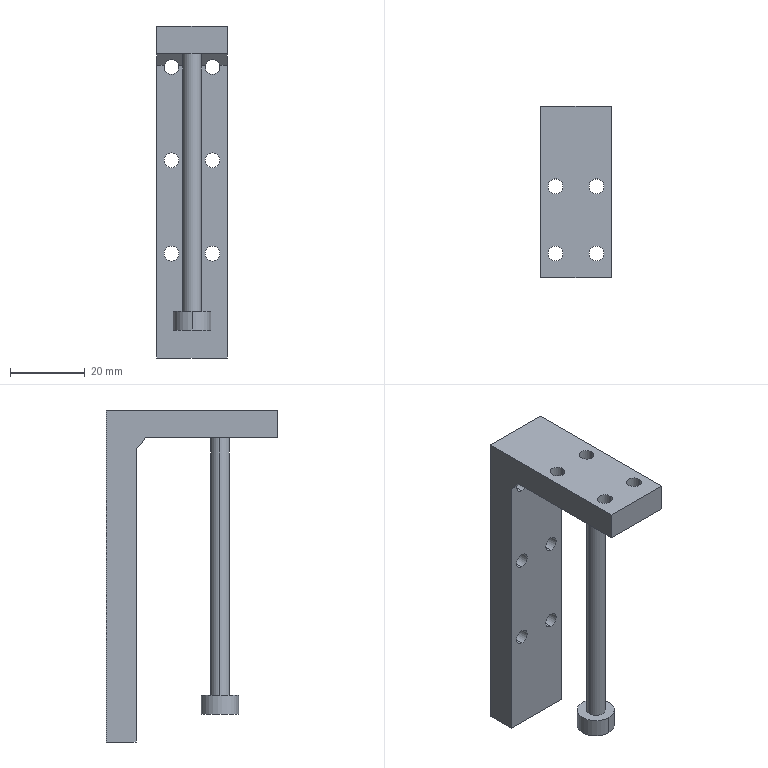Part | NX | 1 solid | 35 faces | box 19 x 46 x 89 mm | volume 19778 mm3 | cylinder 24 | plane 11 | commonest cylinder face diameters 4 x20 5 x2 10 x2
STEP:
#1=CARTESIAN_POINT('',(0.,-5.,-81.5));
#2=VERTEX_POINT('',#1);
#3=CARTESIAN_POINT('',(0.,5.,-81.5));
#4=VERTEX_POINT('',#3);
#5=CARTESIAN_POINT('',(0.,0.,-81.5));
#6=DIRECTION('',(0.,0.,-1.));
#7=DIRECTION('',(0.,1.,0.));
#8=AXIS2_PLACEMENT_3D('',#5,#6,#7);
#9=CIRCLE('',#8,5.);
#10=EDGE_CURVE('',#2,#4,#9,.T.);
#11=ORIENTED_EDGE('',*,*,#10,.F.);
#12=CARTESIAN_POINT('',(0.,-5.,-76.5));
#13=VERTEX_POINT('',#12);
#14=CARTESIAN_POINT('',(0.,-5.,-81.5));
#15=DIRECTION('',(0.,0.,1.));
#16=VECTOR('',#15,1000.);
#17=LINE('',#14,#16);
#18=EDGE_CURVE('',#13,#2,#17,.F.);
#19=ORIENTED_EDGE('',*,*,#18,.F.);
#20=CARTESIAN_POINT('',(0.,5.,-76.5));
#21=VERTEX_POINT('',#20);
#22=CARTESIAN_POINT('',(0.,0.,-76.5));
#23=DIRECTION('',(0.,0.,-1.));
#24=DIRECTION('',(0.,1.,0.));
#25=AXIS2_PLACEMENT_3D('',#22,#23,#24);
#26=CIRCLE('',#25,5.);
#27=EDGE_CURVE('',#13,#21,#26,.T.);
#28=ORIENTED_EDGE('',*,*,#27,.T.);
#29=CARTESIAN_POINT('',(0.,5.,-81.5));
#30=DIRECTION('',(0.,0.,1.));
#31=VECTOR('',#30,1000.);
#32=LINE('',#29,#31);
#33=EDGE_CURVE('',#21,#4,#32,.F.);
#34=ORIENTED_EDGE('',*,*,#33,.T.);
#35=EDGE_LOOP('',(#11,#19,#28,#34));
#36=FACE_BOUND('',#35,.T.);
#37=CARTESIAN_POINT('',(0.,0.,-81.5));
#38=DIRECTION('',(0.,0.,1.));
#39=DIRECTION('',(0.,-1.,0.));
#40=AXIS2_PLACEMENT_3D('',#37,#38,#39);
#41=CYLINDRICAL_SURFACE('',#40,5.);
#42=ADVANCED_FACE('',(#36),#41,.T.);
#43=CARTESIAN_POINT('',(-5.5,30.5,-59.));
#44=VERTEX_POINT('',#43);
#45=CARTESIAN_POINT('',(-5.5,30.5,-63.));
#46=VERTEX_POINT('',#45);
#47=CARTESIAN_POINT('',(-5.5,30.5,-61.));
#48=DIRECTION('',(0.,1.,0.));
#49=DIRECTION('',(0.,0.,1.));
#50=AXIS2_PLACEMENT_3D('',#47,#48,#49);
#51=CIRCLE('',#50,2.);
#52=EDGE_CURVE('',#44,#46,#51,.T.);
#53=ORIENTED_EDGE('',*,*,#52,.T.);
#54=CARTESIAN_POINT('',(-5.5,22.5,-63.));
#55=VERTEX_POINT('',#54);
#56=CARTESIAN_POINT('',(-5.5,-15.5,-63.));
#57=DIRECTION('',(0.,1.,0.));
#58=VECTOR('',#57,1000.);
#59=LINE('',#56,#58);
#60=EDGE_CURVE('',#46,#55,#59,.F.);
#61=ORIENTED_EDGE('',*,*,#60,.T.);
#62=CARTESIAN_POINT('',(-5.5,22.5,-59.));
#63=VERTEX_POINT('',#62);
#64=CARTESIAN_POINT('',(-5.5,22.5,-61.));
#65=DIRECTION('',(0.,1.,0.));
#66=DIRECTION('',(0.,0.,1.));
#67=AXIS2_PLACEMENT_3D('',#64,#65,#66);
#68=CIRCLE('',#67,2.);
#69=EDGE_CURVE('',#63,#55,#68,.T.);
#70=ORIENTED_EDGE('',*,*,#69,.F.);
#71=CARTESIAN_POINT('',(-5.5,-15.5,-59.));
#72=DIRECTION('',(0.,1.,0.));
#73=VECTOR('',#72,1000.);
#74=LINE('',#71,#73);
#75=EDGE_CURVE('',#44,#63,#74,.F.);
#76=ORIENTED_EDGE('',*,*,#75,.F.);
#77=EDGE_LOOP('',(#53,#61,#70,#76));
#78=FACE_BOUND('',#77,.T.);
#79=CARTESIAN_POINT('',(-5.5,-15.5,-61.));
#80=DIRECTION('',(0.,1.,0.));
#81=DIRECTION('',(0.,0.,1.));
#82=AXIS2_PLACEMENT_3D('',#79,#80,#81);
#83=CYLINDRICAL_SURFACE('',#82,2.);
#84=ADVANCED_FACE('',(#78),#83,.F.);
#85=CARTESIAN_POINT('',(5.5,30.5,-63.));
#86=VERTEX_POINT('',#85);
#87=CARTESIAN_POINT('',(5.5,30.5,-59.));
#88=VERTEX_POINT('',#87);
#89=CARTESIAN_POINT('',(5.5,30.5,-61.));
#90=DIRECTION('',(0.,1.,0.));
#91=DIRECTION('',(0.,0.,1.));
#92=AXIS2_PLACEMENT_3D('',#89,#90,#91);
#93=CIRCLE('',#92,2.);
#94=EDGE_CURVE('',#86,#88,#93,.T.);
#95=ORIENTED_EDGE('',*,*,#94,.T.);
#96=CARTESIAN_POINT('',(5.5,22.5,-59.));
#97=VERTEX_POINT('',#96);
#98=CARTESIAN_POINT('',(5.5,-15.5,-59.));
#99=DIRECTION('',(0.,1.,0.));
#100=VECTOR('',#99,1000.);
#101=LINE('',#98,#100);
#102=EDGE_CURVE('',#97,#88,#101,.T.);
#103=ORIENTED_EDGE('',*,*,#102,.F.);
#104=CARTESIAN_POINT('',(5.5,22.5,-63.));
#105=VERTEX_POINT('',#104);
#106=CARTESIAN_POINT('',(5.5,22.5,-61.));
#107=DIRECTION('',(0.,1.,0.));
#108=DIRECTION('',(0.,0.,1.));
#109=AXIS2_PLACEMENT_3D('',#106,#107,#108);
#110=CIRCLE('',#109,2.);
#111=EDGE_CURVE('',#105,#97,#110,.T.);
#112=ORIENTED_EDGE('',*,*,#111,.F.);
#113=CARTESIAN_POINT('',(5.5,-15.5,-63.));
#114=DIRECTION('',(0.,1.,0.));
#115=VECTOR('',#114,1000.);
#116=LINE('',#113,#115);
#117=EDGE_CURVE('',#105,#86,#116,.T.);
#118=ORIENTED_EDGE('',*,*,#117,.T.);
#119=EDGE_LOOP('',(#95,#103,#112,#118));
#120=FACE_BOUND('',#119,.T.);
#121=CARTESIAN_POINT('',(5.5,-15.5,-61.));
#122=DIRECTION('',(0.,1.,0.));
#123=DIRECTION('',(0.,0.,1.));
#124=AXIS2_PLACEMENT_3D('',#121,#122,#123);
#125=CYLINDRICAL_SURFACE('',#124,2.);
#126=ADVANCED_FACE('',(#120),#125,.F.);
#127=CARTESIAN_POINT('',(5.5,22.5,-13.));
#128=VERTEX_POINT('',#127);
#129=CARTESIAN_POINT('',(3.564,22.5,-10.5));
#130=VERTEX_POINT('',#129);
#131=CARTESIAN_POINT('',(5.5,22.5,-11.));
#132=DIRECTION('',(0.,1.,0.));
#133=DIRECTION('',(0.,0.,1.));
#134=AXIS2_PLACEMENT_3D('',#131,#132,#133);
#135=CIRCLE('',#134,2.);
#136=EDGE_CURVE('',#128,#130,#135,.T.);
#137=ORIENTED_EDGE('',*,*,#136,.F.);
#138=CARTESIAN_POINT('',(5.5,30.5,-13.));
#139=VERTEX_POINT('',#138);
#140=CARTESIAN_POINT('',(5.5,-15.5,-13.));
#141=DIRECTION('',(0.,1.,0.));
#142=VECTOR('',#141,1000.);
#143=LINE('',#140,#142);
#144=EDGE_CURVE('',#139,#128,#143,.F.);
#145=ORIENTED_EDGE('',*,*,#144,.F.);
#146=CARTESIAN_POINT('',(5.5,30.5,-9.));
#147=VERTEX_POINT('',#146);
#148=CARTESIAN_POINT('',(5.5,30.5,-11.));
#149=DIRECTION('',(0.,1.,0.));
#150=DIRECTION('',(0.,0.,-1.));
#151=AXIS2_PLACEMENT_3D('',#148,#149,#150);
#152=CIRCLE('',#151,2.);
#153=EDGE_CURVE('',#139,#147,#152,.T.);
#154=ORIENTED_EDGE('',*,*,#153,.T.);
#155=CARTESIAN_POINT('',(5.5,21.241,-9.));
#156=VERTEX_POINT('',#155);
#157=CARTESIAN_POINT('',(5.5,-15.5,-9.));
#158=DIRECTION('',(0.,1.,0.));
#159=VECTOR('',#158,1000.);
#160=LINE('',#157,#159);
#161=EDGE_CURVE('',#147,#156,#160,.F.);
#162=ORIENTED_EDGE('',*,*,#161,.T.);
#163=CARTESIAN_POINT('',(3.564,22.5,-10.5));
#164=CARTESIAN_POINT('',(3.801,21.729,-9.581));
#165=CARTESIAN_POINT('',(4.551,21.241,-9.));
#166=CARTESIAN_POINT('',(5.5,21.241,-9.));
#167=(BOUNDED_CURVE()B_SPLINE_CURVE(3,(#163,#164,#165,#166),.UNSPECIFIED.,.F.,.F.)B_SPLINE_CURVE_WITH_KNOTS((4,4),(1.823,3.142),.UNSPECIFIED.)CURVE()GEOMETRIC_REPRESENTATION_ITEM()RATIONAL_B_SPLINE_CURVE((1.,0.8604,0.8604,1.))REPRESENTATION_ITEM(''));
#168=EDGE_CURVE('',#130,#156,#167,.T.);
#169=ORIENTED_EDGE('',*,*,#168,.F.);
#170=EDGE_LOOP('',(#137,#145,#154,#162,#169));
#171=FACE_BOUND('',#170,.T.);
#172=CARTESIAN_POINT('',(5.5,-15.5,-11.));
#173=DIRECTION('',(0.,1.,0.));
#174=DIRECTION('',(0.,0.,1.));
#175=AXIS2_PLACEMENT_3D('',#172,#173,#174);
#176=CYLINDRICAL_SURFACE('',#175,2.);
#177=ADVANCED_FACE('',(#171),#176,.F.);
#178=CARTESIAN_POINT('',(-5.5,22.5,-38.));
#179=VERTEX_POINT('',#178);
#180=CARTESIAN_POINT('',(-5.5,22.5,-34.));
#181=VERTEX_POINT('',#180);
#182=CARTESIAN_POINT('',(-5.5,22.5,-36.));
#183=DIRECTION('',(0.,1.,0.));
#184=DIRECTION('',(0.,0.,1.));
#185=AXIS2_PLACEMENT_3D('',#182,#183,#184);
#186=CIRCLE('',#185,2.);
#187=EDGE_CURVE('',#179,#181,#186,.T.);
#188=ORIENTED_EDGE('',*,*,#187,.F.);
#189=CARTESIAN_POINT('',(-5.5,30.5,-38.));
#190=VERTEX_POINT('',#189);
#191=CARTESIAN_POINT('',(-5.5,-15.5,-38.));
#192=DIRECTION('',(0.,1.,0.));
#193=VECTOR('',#192,1000.);
#194=LINE('',#191,#193);
#195=EDGE_CURVE('',#190,#179,#194,.F.);
#196=ORIENTED_EDGE('',*,*,#195,.F.);
#197=CARTESIAN_POINT('',(-5.5,30.5,-34.));
#198=VERTEX_POINT('',#197);
#199=CARTESIAN_POINT('',(-5.5,30.5,-36.));
#200=DIRECTION('',(0.,1.,0.));
#201=DIRECTION('',(0.,0.,1.));
#202=AXIS2_PLACEMENT_3D('',#199,#200,#201);
#203=CIRCLE('',#202,2.);
#204=EDGE_CURVE('',#190,#198,#203,.T.);
#205=ORIENTED_EDGE('',*,*,#204,.T.);
#206=CARTESIAN_POINT('',(-5.5,-15.5,-34.));
#207=DIRECTION('',(0.,1.,0.));
#208=VECTOR('',#207,1000.);
#209=LINE('',#206,#208);
#210=EDGE_CURVE('',#198,#181,#209,.F.);
#211=ORIENTED_EDGE('',*,*,#210,.T.);
#212=EDGE_LOOP('',(#188,#196,#205,#211));
#213=FACE_BOUND('',#212,.T.);
#214=CARTESIAN_POINT('',(-5.5,-15.5,-36.));
#215=DIRECTION('',(0.,1.,0.));
#216=DIRECTION('',(0.,0.,1.));
#217=AXIS2_PLACEMENT_3D('',#214,#215,#216);
#218=CYLINDRICAL_SURFACE('',#217,2.);
#219=ADVANCED_FACE('',(#213),#218,.F.);
#220=CARTESIAN_POINT('',(-5.5,22.5,-13.));
#221=VERTEX_POINT('',#220);
#222=CARTESIAN_POINT('',(-7.436,22.5,-10.5));
#223=VERTEX_POINT('',#222);
#224=CARTESIAN_POINT('',(-5.5,22.5,-11.));
#225=DIRECTION('',(0.,1.,0.));
#226=DIRECTION('',(0.,0.,1.));
#227=AXIS2_PLACEMENT_3D('',#224,#225,#226);
#228=CIRCLE('',#227,2.);
#229=EDGE_CURVE('',#221,#223,#228,.T.);
#230=ORIENTED_EDGE('',*,*,#229,.F.);
#231=CARTESIAN_POINT('',(-5.5,30.5,-13.));
#232=VERTEX_POINT('',#231);
#233=CARTESIAN_POINT('',(-5.5,-15.5,-13.));
#234=DIRECTION('',(0.,1.,0.));
#235=VECTOR('',#234,1000.);
#236=LINE('',#233,#235);
#237=EDGE_CURVE('',#232,#221,#236,.F.);
#238=ORIENTED_EDGE('',*,*,#237,.F.);
#239=CARTESIAN_POINT('',(-5.5,30.5,-9.));
#240=VERTEX_POINT('',#239);
#241=CARTESIAN_POINT('',(-5.5,30.5,-11.));
#242=DIRECTION('',(0.,1.,0.));
#243=DIRECTION('',(0.,0.,1.));
#244=AXIS2_PLACEMENT_3D('',#241,#242,#243);
#245=CIRCLE('',#244,2.);
#246=EDGE_CURVE('',#232,#240,#245,.T.);
#247=ORIENTED_EDGE('',*,*,#246,.T.);
#248=CARTESIAN_POINT('',(-5.5,21.241,-9.));
#249=VERTEX_POINT('',#248);
#250=CARTESIAN_POINT('',(-5.5,-15.5,-9.));
#251=DIRECTION('',(0.,1.,0.));
#252=VECTOR('',#251,1000.);
#253=LINE('',#250,#252);
#254=EDGE_CURVE('',#240,#249,#253,.F.);
#255=ORIENTED_EDGE('',*,*,#254,.T.);
#256=CARTESIAN_POINT('',(-7.436,22.5,-10.5));
#257=CARTESIAN_POINT('',(-7.199,21.729,-9.581));
#258=CARTESIAN_POINT('',(-6.449,21.241,-9.));
#259=CARTESIAN_POINT('',(-5.5,21.241,-9.));
#260=(BOUNDED_CURVE()B_SPLINE_CURVE(3,(#256,#257,#258,#259),.UNSPECIFIED.,.F.,.F.)B_SPLINE_CURVE_WITH_KNOTS((4,4),(1.823,3.142),.UNSPECIFIED.)CURVE()GEOMETRIC_REPRESENTATION_ITEM()RATIONAL_B_SPLINE_CURVE((1.,0.8604,0.8604,1.))REPRESENTATION_ITEM(''));
#261=EDGE_CURVE('',#223,#249,#260,.T.);
#262=ORIENTED_EDGE('',*,*,#261,.F.);
#263=EDGE_LOOP('',(#230,#238,#247,#255,#262));
#264=FACE_BOUND('',#263,.T.);
#265=CARTESIAN_POINT('',(-5.5,-15.5,-11.));
#266=DIRECTION('',(0.,1.,0.));
#267=DIRECTION('',(0.,0.,1.));
#268=AXIS2_PLACEMENT_3D('',#265,#266,#267);
#269=CYLINDRICAL_SURFACE('',#268,2.);
#270=ADVANCED_FACE('',(#264),#269,.F.);
#271=CARTESIAN_POINT('',(5.5,30.5,-38.));
#272=VERTEX_POINT('',#271);
#273=CARTESIAN_POINT('',(5.5,30.5,-34.));
#274=VERTEX_POINT('',#273);
#275=CARTESIAN_POINT('',(5.5,30.5,-36.));
#276=DIRECTION('',(0.,1.,0.));
#277=DIRECTION('',(0.,0.,-1.));
#278=AXIS2_PLACEMENT_3D('',#275,#276,#277);
#279=CIRCLE('',#278,2.);
#280=EDGE_CURVE('',#272,#274,#279,.T.);
#281=ORIENTED_EDGE('',*,*,#280,.T.);
#282=CARTESIAN_POINT('',(5.5,22.5,-34.));
#283=VERTEX_POINT('',#282);
#284=CARTESIAN_POINT('',(5.5,-15.5,-34.));
#285=DIRECTION('',(0.,1.,0.));
#286=VECTOR('',#285,1000.);
#287=LINE('',#284,#286);
#288=EDGE_CURVE('',#283,#274,#287,.T.);
#289=ORIENTED_EDGE('',*,*,#288,.F.);
#290=CARTESIAN_POINT('',(5.5,22.5,-38.));
#291=VERTEX_POINT('',#290);
#292=CARTESIAN_POINT('',(5.5,22.5,-36.));
#293=DIRECTION('',(0.,1.,0.));
#294=DIRECTION('',(0.,0.,1.));
#295=AXIS2_PLACEMENT_3D('',#292,#293,#294);
#296=CIRCLE('',#295,2.);
#297=EDGE_CURVE('',#291,#283,#296,.T.);
#298=ORIENTED_EDGE('',*,*,#297,.F.);
#299=CARTESIAN_POINT('',(5.5,-15.5,-38.));
#300=DIRECTION('',(0.,1.,0.));
#301=VECTOR('',#300,1000.);
#302=LINE('',#299,#301);
#303=EDGE_CURVE('',#291,#272,#302,.T.);
#304=ORIENTED_EDGE('',*,*,#303,.T.);
#305=EDGE_LOOP('',(#281,#289,#298,#304));
#306=FACE_BOUND('',#305,.T.);
#307=CARTESIAN_POINT('',(5.5,-15.5,-36.));
#308=DIRECTION('',(0.,1.,0.));
#309=DIRECTION('',(0.,0.,1.));
#310=AXIS2_PLACEMENT_3D('',#307,#308,#309);
#311=CYLINDRICAL_SURFACE('',#310,2.);
#312=ADVANCED_FACE('',(#306),#311,.F.);
#313=CARTESIAN_POINT('',(3.5,-9.,-7.5));
#314=VERTEX_POINT('',#313);
#315=CARTESIAN_POINT('',(7.5,-9.,-7.5));
#316=VERTEX_POINT('',#315);
#317=CARTESIAN_POINT('',(5.5,-9.,-7.5));
#318=DIRECTION('',(0.,0.,1.));
#319=DIRECTION('',(0.,-1.,0.));
#320=AXIS2_PLACEMENT_3D('',#317,#318,#319);
#321=CIRCLE('',#320,2.);
#322=EDGE_CURVE('',#314,#316,#321,.T.);
#323=ORIENTED_EDGE('',*,*,#322,.F.);
#324=CARTESIAN_POINT('',(3.5,-9.,0.));
#325=VERTEX_POINT('',#324);
#326=CARTESIAN_POINT('',(3.5,-9.,-89.));
#327=DIRECTION('',(0.,0.,1.));
#328=VECTOR('',#327,1000.);
#329=LINE('',#326,#328);
#330=EDGE_CURVE('',#314,#325,#329,.T.);
#331=ORIENTED_EDGE('',*,*,#330,.T.);
#332=CARTESIAN_POINT('',(7.5,-9.,0.));
#333=VERTEX_POINT('',#332);
#334=CARTESIAN_POINT('',(5.5,-9.,0.));
#335=DIRECTION('',(0.,0.,1.));
#336=DIRECTION('',(-1.,0.,0.));
#337=AXIS2_PLACEMENT_3D('',#334,#335,#336);
#338=CIRCLE('',#337,2.);
#339=EDGE_CURVE('',#325,#333,#338,.T.);
#340=ORIENTED_EDGE('',*,*,#339,.T.);
#341=CARTESIAN_POINT('',(7.5,-9.,-89.));
#342=DIRECTION('',(0.,0.,1.));
#343=VECTOR('',#342,1000.);
#344=LINE('',#341,#343);
#345=EDGE_CURVE('',#316,#333,#344,.T.);
#346=ORIENTED_EDGE('',*,*,#345,.F.);
#347=EDGE_LOOP('',(#323,#331,#340,#346));
#348=FACE_BOUND('',#347,.T.);
#349=CARTESIAN_POINT('',(5.5,-9.,-89.));
#350=DIRECTION('',(0.,0.,1.));
#351=DIRECTION('',(1.,0.,0.));
#352=AXIS2_PLACEMENT_3D('',#349,#350,#351);
#353=CYLINDRICAL_SURFACE('',#352,2.);
#354=ADVANCED_FACE('',(#348),#353,.F.);
#355=CARTESIAN_POINT('',(-7.5,-9.,-7.5));
#356=VERTEX_POINT('',#355);
#357=CARTESIAN_POINT('',(-3.5,-9.,-7.5));
#358=VERTEX_POINT('',#357);
#359=CARTESIAN_POINT('',(-5.5,-9.,-7.5));
#360=DIRECTION('',(0.,0.,1.));
#361=DIRECTION('',(0.,-1.,0.));
#362=AXIS2_PLACEMENT_3D('',#359,#360,#361);
#363=CIRCLE('',#362,2.);
#364=EDGE_CURVE('',#356,#358,#363,.T.);
#365=ORIENTED_EDGE('',*,*,#364,.F.);
#366=CARTESIAN_POINT('',(-7.5,-9.,0.));
#367=VERTEX_POINT('',#366);
#368=CARTESIAN_POINT('',(-7.5,-9.,-89.));
#369=DIRECTION('',(0.,0.,1.));
#370=VECTOR('',#369,1000.);
#371=LINE('',#368,#370);
#372=EDGE_CURVE('',#367,#356,#371,.F.);
#373=ORIENTED_EDGE('',*,*,#372,.F.);
#374=CARTESIAN_POINT('',(-3.5,-9.,0.));
#375=VERTEX_POINT('',#374);
#376=CARTESIAN_POINT('',(-5.5,-9.,0.));
#377=DIRECTION('',(0.,0.,1.));
#378=DIRECTION('',(1.,0.,0.));
#379=AXIS2_PLACEMENT_3D('',#376,#377,#378);
#380=CIRCLE('',#379,2.);
#381=EDGE_CURVE('',#367,#375,#380,.T.);
#382=ORIENTED_EDGE('',*,*,#381,.T.);
#383=CARTESIAN_POINT('',(-3.5,-9.,-89.));
#384=DIRECTION('',(0.,0.,1.));
#385=VECTOR('',#384,1000.);
#386=LINE('',#383,#385);
#387=EDGE_CURVE('',#375,#358,#386,.F.);
#388=ORIENTED_EDGE('',*,*,#387,.T.);
#389=EDGE_LOOP('',(#365,#373,#382,#388));
#390=FACE_BOUND('',#389,.T.);
#391=CARTESIAN_POINT('',(-5.5,-9.,-89.));
#392=DIRECTION('',(0.,0.,1.));
#393=DIRECTION('',(1.,0.,0.));
#394=AXIS2_PLACEMENT_3D('',#391,#392,#393);
#395=CYLINDRICAL_SURFACE('',#394,2.);
#396=ADVANCED_FACE('',(#390),#395,.F.);
#397=CARTESIAN_POINT('',(-3.5,9.,-7.5));
#398=VERTEX_POINT('',#397);
#399=CARTESIAN_POINT('',(-7.5,9.,-7.5));
#400=VERTEX_POINT('',#399);
#401=CARTESIAN_POINT('',(-5.5,9.,-7.5));
#402=DIRECTION('',(0.,0.,1.));
#403=DIRECTION('',(0.,-1.,0.));
#404=AXIS2_PLACEMENT_3D('',#401,#402,#403);
#405=CIRCLE('',#404,2.);
#406=EDGE_CURVE('',#398,#400,#405,.T.);
#407=ORIENTED_EDGE('',*,*,#406,.F.);
#408=CARTESIAN_POINT('',(-3.5,9.,0.));
#409=VERTEX_POINT('',#408);
#410=CARTESIAN_POINT('',(-3.5,9.,-89.));
#411=DIRECTION('',(0.,0.,1.));
#412=VECTOR('',#411,1000.);
#413=LINE('',#410,#412);
#414=EDGE_CURVE('',#398,#409,#413,.T.);
#415=ORIENTED_EDGE('',*,*,#414,.T.);
#416=CARTESIAN_POINT('',(-7.5,9.,0.));
#417=VERTEX_POINT('',#416);
#418=CARTESIAN_POINT('',(-5.5,9.,0.));
#419=DIRECTION('',(0.,0.,1.));
#420=DIRECTION('',(-1.,0.,0.));
#421=AXIS2_PLACEMENT_3D('',#418,#419,#420);
#422=CIRCLE('',#421,2.);
#423=EDGE_CURVE('',#409,#417,#422,.T.);
#424=ORIENTED_EDGE('',*,*,#423,.T.);
#425=CARTESIAN_POINT('',(-7.5,9.,-89.));
#426=DIRECTION('',(0.,0.,1.));
#427=VECTOR('',#426,1000.);
#428=LINE('',#425,#427);
#429=EDGE_CURVE('',#400,#417,#428,.T.);
#430=ORIENTED_EDGE('',*,*,#429,.F.);
#431=EDGE_LOOP('',(#407,#415,#424,#430));
#432=FACE_BOUND('',#431,.T.);
#433=CARTESIAN_POINT('',(-5.5,9.,-89.));
#434=DIRECTION('',(0.,0.,1.));
#435=DIRECTION('',(1.,0.,0.));
#436=AXIS2_PLACEMENT_3D('',#433,#434,#435);
#437=CYLINDRICAL_SURFACE('',#436,2.);
#438=ADVANCED_FACE('',(#432),#437,.F.);
#439=CARTESIAN_POINT('',(3.5,9.,0.));
#440=VERTEX_POINT('',#439);
#441=CARTESIAN_POINT('',(7.5,9.,0.));
#442=VERTEX_POINT('',#441);
#443=CARTESIAN_POINT('',(5.5,9.,0.));
#444=DIRECTION('',(0.,0.,1.));
#445=DIRECTION('',(1.,0.,0.));
#446=AXIS2_PLACEMENT_3D('',#443,#444,#445);
#447=CIRCLE('',#446,2.);
#448=EDGE_CURVE('',#440,#442,#447,.T.);
#449=ORIENTED_EDGE('',*,*,#448,.T.);
#450=CARTESIAN_POINT('',(7.5,9.,-7.5));
#451=VERTEX_POINT('',#450);
#452=CARTESIAN_POINT('',(7.5,9.,-89.));
#453=DIRECTION('',(0.,0.,1.));
#454=VECTOR('',#453,1000.);
#455=LINE('',#452,#454);
#456=EDGE_CURVE('',#451,#442,#455,.T.);
#457=ORIENTED_EDGE('',*,*,#456,.F.);
#458=CARTESIAN_POINT('',(3.5,9.,-7.5));
#459=VERTEX_POINT('',#458);
#460=CARTESIAN_POINT('',(5.5,9.,-7.5));
#461=DIRECTION('',(0.,0.,1.));
#462=DIRECTION('',(0.,-1.,0.));
#463=AXIS2_PLACEMENT_3D('',#460,#461,#462);
#464=CIRCLE('',#463,2.);
#465=EDGE_CURVE('',#459,#451,#464,.T.);
#466=ORIENTED_EDGE('',*,*,#465,.F.);
#467=CARTESIAN_POINT('',(3.5,9.,-89.));
#468=DIRECTION('',(0.,0.,1.));
#469=VECTOR('',#468,1000.);
#470=LINE('',#467,#469);
#471=EDGE_CURVE('',#459,#440,#470,.T.);
#472=ORIENTED_EDGE('',*,*,#471,.T.);
#473=EDGE_LOOP('',(#449,#457,#466,#472));
#474=FACE_BOUND('',#473,.T.);
#475=CARTESIAN_POINT('',(5.5,9.,-89.));
#476=DIRECTION('',(0.,0.,1.));
#477=DIRECTION('',(1.,0.,0.));
#478=AXIS2_PLACEMENT_3D('',#475,#476,#477);
#479=CYLINDRICAL_SURFACE('',#478,2.);
#480=ADVANCED_FACE('',(#474),#479,.F.);
#481=CARTESIAN_POINT('',(-2.5,0.,-76.5));
#482=VERTEX_POINT('',#481);
#483=CARTESIAN_POINT('',(2.5,0.,-76.5));
#484=VERTEX_POINT('',#483);
#485=CARTESIAN_POINT('',(0.,0.,-76.5));
#486=DIRECTION('',(0.,0.,-1.));
#487=DIRECTION('',(0.,1.,0.));
#488=AXIS2_PLACEMENT_3D('',#485,#486,#487);
#489=CIRCLE('',#488,2.5);
#490=EDGE_CURVE('',#482,#484,#489,.T.);
#491=ORIENTED_EDGE('',*,*,#490,.F.);
#492=CARTESIAN_POINT('',(-2.5,0.,-7.5));
#493=VERTEX_POINT('',#492);
#494=CARTESIAN_POINT('',(-2.5,0.,-79.));
#495=DIRECTION('',(0.,0.,1.));
#496=VECTOR('',#495,1000.);
#497=LINE('',#494,#496);
#498=EDGE_CURVE('',#482,#493,#497,.T.);
#499=ORIENTED_EDGE('',*,*,#498,.T.);
#500=CARTESIAN_POINT('',(2.5,0.,-7.5));
#501=VERTEX_POINT('',#500);
#502=CARTESIAN_POINT('',(0.,0.,-7.5));
#503=DIRECTION('',(0.,0.,-1.));
#504=DIRECTION('',(0.,-1.,0.));
#505=AXIS2_PLACEMENT_3D('',#502,#503,#504);
#506=CIRCLE('',#505,2.5);
#507=EDGE_CURVE('',#493,#501,#506,.T.);
#508=ORIENTED_EDGE('',*,*,#507,.T.);
#509=CARTESIAN_POINT('',(2.5,0.,-79.));
#510=DIRECTION('',(0.,0.,1.));
#511=VECTOR('',#510,1000.);
#512=LINE('',#509,#511);
#513=EDGE_CURVE('',#484,#501,#512,.T.);
#514=ORIENTED_EDGE('',*,*,#513,.F.);
#515=EDGE_LOOP('',(#491,#499,#508,#514));
#516=FACE_BOUND('',#515,.T.);
#517=CARTESIAN_POINT('',(0.,0.,-79.));
#518=DIRECTION('',(0.,0.,1.));
#519=DIRECTION('',(1.,0.,0.));
#520=AXIS2_PLACEMENT_3D('',#517,#518,#519);
#521=CYLINDRICAL_SURFACE('',#520,2.5);
#522=ADVANCED_FACE('',(#516),#521,.T.);
#523=ORIENTED_EDGE('',*,*,#10,.T.);
#524=CARTESIAN_POINT('',(0.,0.,-81.5));
#525=DIRECTION('',(0.,0.,-1.));
#526=DIRECTION('',(0.,1.,0.));
#527=AXIS2_PLACEMENT_3D('',#524,#525,#526);
#528=CIRCLE('',#527,5.);
#529=EDGE_CURVE('',#4,#2,#528,.T.);
#530=ORIENTED_EDGE('',*,*,#529,.T.);
#531=EDGE_LOOP('',(#523,#530));
#532=FACE_BOUND('',#531,.T.);
#533=CARTESIAN_POINT('',(0.,0.,-81.5));
#534=DIRECTION('',(0.,0.,-1.));
#535=DIRECTION('',(-1.,0.,0.));
#536=AXIS2_PLACEMENT_3D('',#533,#534,#535);
#537=PLANE('',#536);
#538=ADVANCED_FACE('',(#532),#537,.T.);
#539=CARTESIAN_POINT('',(-9.5,-15.5,-7.5));
#540=VERTEX_POINT('',#539);
#541=CARTESIAN_POINT('',(-9.5,19.983,-7.5));
#542=VERTEX_POINT('',#541);
#543=CARTESIAN_POINT('',(-9.5,19.983,-7.5));
#544=DIRECTION('',(0.,1.,0.));
#545=VECTOR('',#544,1000.);
#546=LINE('',#543,#545);
#547=EDGE_CURVE('',#540,#542,#546,.T.);
#548=ORIENTED_EDGE('',*,*,#547,.T.);
#549=CARTESIAN_POINT('',(9.5,19.983,-7.5));
#550=VERTEX_POINT('',#549);
#551=CARTESIAN_POINT('',(9.5,19.983,-7.5));
#552=DIRECTION('',(-1.,0.,0.));
#553=VECTOR('',#552,1000.);
#554=LINE('',#551,#553);
#555=EDGE_CURVE('',#550,#542,#554,.T.);
#556=ORIENTED_EDGE('',*,*,#555,.F.);
#557=CARTESIAN_POINT('',(9.5,-15.5,-7.5));
#558=VERTEX_POINT('',#557);
#559=CARTESIAN_POINT('',(9.5,19.983,-7.5));
#560=DIRECTION('',(0.,1.,0.));
#561=VECTOR('',#560,1000.);
#562=LINE('',#559,#561);
#563=EDGE_CURVE('',#558,#550,#562,.T.);
#564=ORIENTED_EDGE('',*,*,#563,.F.);
#565=CARTESIAN_POINT('',(9.5,-15.5,-7.5));
#566=DIRECTION('',(-1.,0.,0.));
#567=VECTOR('',#566,1000.);
#568=LINE('',#565,#567);
#569=EDGE_CURVE('',#558,#540,#568,.T.);
#570=ORIENTED_EDGE('',*,*,#569,.T.);
#571=EDGE_LOOP('',(#548,#556,#564,#570));
#572=FACE_BOUND('',#571,.T.);
#573=CARTESIAN_POINT('',(5.5,9.,-7.5));
#574=DIRECTION('',(0.,0.,1.));
#575=DIRECTION('',(0.,-1.,0.));
#576=AXIS2_PLACEMENT_3D('',#573,#574,#575);
#577=CIRCLE('',#576,2.);
#578=EDGE_CURVE('',#451,#459,#577,.T.);
#579=ORIENTED_EDGE('',*,*,#578,.T.);
#580=ORIENTED_EDGE('',*,*,#465,.T.);
#581=EDGE_LOOP('',(#579,#580));
#582=FACE_BOUND('',#581,.T.);
#583=ORIENTED_EDGE('',*,*,#406,.T.);
#584=CARTESIAN_POINT('',(-5.5,9.,-7.5));
#585=DIRECTION('',(0.,0.,1.));
#586=DIRECTION('',(0.,-1.,0.));
#587=AXIS2_PLACEMENT_3D('',#584,#585,#586);
#588=CIRCLE('',#587,2.);
#589=EDGE_CURVE('',#400,#398,#588,.T.);
#590=ORIENTED_EDGE('',*,*,#589,.T.);
#591=EDGE_LOOP('',(#583,#590));
#592=FACE_BOUND('',#591,.T.);
#593=ORIENTED_EDGE('',*,*,#364,.T.);
#594=CARTESIAN_POINT('',(-5.5,-9.,-7.5));
#595=DIRECTION('',(0.,0.,1.));
#596=DIRECTION('',(0.,-1.,0.));
#597=AXIS2_PLACEMENT_3D('',#594,#595,#596);
#598=CIRCLE('',#597,2.);
#599=EDGE_CURVE('',#358,#356,#598,.T.);
#600=ORIENTED_EDGE('',*,*,#599,.T.);
#601=EDGE_LOOP('',(#593,#600));
#602=FACE_BOUND('',#601,.T.);
#603=ORIENTED_EDGE('',*,*,#322,.T.);
#604=CARTESIAN_POINT('',(5.5,-9.,-7.5));
#605=DIRECTION('',(0.,0.,1.));
#606=DIRECTION('',(0.,-1.,0.));
#607=AXIS2_PLACEMENT_3D('',#604,#605,#606);
#608=CIRCLE('',#607,2.);
#609=EDGE_CURVE('',#316,#314,#608,.T.);
#610=ORIENTED_EDGE('',*,*,#609,.T.);
#611=EDGE_LOOP('',(#603,#610));
#612=FACE_BOUND('',#611,.T.);
#613=ORIENTED_EDGE('',*,*,#507,.F.);
#614=CARTESIAN_POINT('',(0.,0.,-7.5));
#615=DIRECTION('',(0.,0.,-1.));
#616=DIRECTION('',(0.,-1.,0.));
#617=AXIS2_PLACEMENT_3D('',#614,#615,#616);
#618=CIRCLE('',#617,2.5);
#619=EDGE_CURVE('',#501,#493,#618,.T.);
#620=ORIENTED_EDGE('',*,*,#619,.F.);
#621=EDGE_LOOP('',(#613,#620));
#622=FACE_BOUND('',#621,.T.);
#623=CARTESIAN_POINT('',(9.5,19.983,-7.5));
#624=DIRECTION('',(0.,0.,1.));
#625=DIRECTION('',(0.,-1.,0.));
#626=AXIS2_PLACEMENT_3D('',#623,#624,#625);
#627=PLANE('',#626);
#628=ADVANCED_FACE('',(#572,#582,#592,#602,#612,#622),#627,.F.);
#629=CARTESIAN_POINT('',(-9.5,-15.5,0.));
#630=VERTEX_POINT('',#629);
#631=CARTESIAN_POINT('',(-9.5,-15.5,-7.5));
#632=DIRECTION('',(0.,0.,-1.));
#633=VECTOR('',#632,1000.);
#634=LINE('',#631,#633);
#635=EDGE_CURVE('',#630,#540,#634,.T.);
#636=ORIENTED_EDGE('',*,*,#635,.T.);
#637=ORIENTED_EDGE('',*,*,#569,.F.);
#638=CARTESIAN_POINT('',(9.5,-15.5,0.));
#639=VERTEX_POINT('',#638);
#640=CARTESIAN_POINT('',(9.5,-15.5,-7.5));
#641=DIRECTION('',(0.,0.,-1.));
#642=VECTOR('',#641,1000.);
#643=LINE('',#640,#642);
#644=EDGE_CURVE('',#639,#558,#643,.T.);
#645=ORIENTED_EDGE('',*,*,#644,.F.);
#646=CARTESIAN_POINT('',(9.5,-15.5,0.));
#647=DIRECTION('',(-1.,0.,0.));
#648=VECTOR('',#647,1000.);
#649=LINE('',#646,#648);
#650=EDGE_CURVE('',#639,#630,#649,.T.);
#651=ORIENTED_EDGE('',*,*,#650,.T.);
#652=EDGE_LOOP('',(#636,#637,#645,#651));
#653=FACE_BOUND('',#652,.T.);
#654=CARTESIAN_POINT('',(9.5,-15.5,-7.5));
#655=DIRECTION('',(0.,1.,0.));
#656=DIRECTION('',(1.,0.,0.));
#657=AXIS2_PLACEMENT_3D('',#654,#655,#656);
#658=PLANE('',#657);
#659=ADVANCED_FACE('',(#653),#658,.F.);
#660=CARTESIAN_POINT('',(-3.564,22.5,-10.5));
#661=VERTEX_POINT('',#660);
#662=CARTESIAN_POINT('',(9.5,22.5,-10.5));
#663=DIRECTION('',(-1.,0.,0.));
#664=VECTOR('',#663,1000.);
#665=LINE('',#662,#664);
#666=EDGE_CURVE('',#130,#661,#665,.T.);
#667=ORIENTED_EDGE('',*,*,#666,.F.);
#668=ORIENTED_EDGE('',*,*,#168,.T.);
#669=CARTESIAN_POINT('',(7.436,22.5,-10.5));
#670=VERTEX_POINT('',#669);
#671=CARTESIAN_POINT('',(5.5,21.241,-9.));
#672=CARTESIAN_POINT('',(6.449,21.241,-9.));
#673=CARTESIAN_POINT('',(7.199,21.729,-9.581));
#674=CARTESIAN_POINT('',(7.436,22.5,-10.5));
#675=(BOUNDED_CURVE()B_SPLINE_CURVE(3,(#671,#672,#673,#674),.UNSPECIFIED.,.F.,.F.)B_SPLINE_CURVE_WITH_KNOTS((4,4),(3.142,4.46),.UNSPECIFIED.)CURVE()GEOMETRIC_REPRESENTATION_ITEM()RATIONAL_B_SPLINE_CURVE((1.,0.8604,0.8604,1.))REPRESENTATION_ITEM(''));
#676=EDGE_CURVE('',#156,#670,#675,.T.);
#677=ORIENTED_EDGE('',*,*,#676,.T.);
#678=CARTESIAN_POINT('',(9.5,22.5,-10.5));
#679=VERTEX_POINT('',#678);
#680=CARTESIAN_POINT('',(9.5,22.5,-10.5));
#681=DIRECTION('',(-1.,0.,0.));
#682=VECTOR('',#681,1000.);
#683=LINE('',#680,#682);
#684=EDGE_CURVE('',#679,#670,#683,.T.);
#685=ORIENTED_EDGE('',*,*,#684,.F.);
#686=CARTESIAN_POINT('',(9.5,22.5,-10.5));
#687=DIRECTION('',(0.,0.6428,-0.766));
#688=VECTOR('',#687,1000.);
#689=LINE('',#686,#688);
#690=EDGE_CURVE('',#550,#679,#689,.T.);
#691=ORIENTED_EDGE('',*,*,#690,.F.);
#692=ORIENTED_EDGE('',*,*,#555,.T.);
#693=CARTESIAN_POINT('',(-9.5,22.5,-10.5));
#694=VERTEX_POINT('',#693);
#695=CARTESIAN_POINT('',(-9.5,22.5,-10.5));
#696=DIRECTION('',(0.,0.6428,-0.766));
#697=VECTOR('',#696,1000.);
#698=LINE('',#695,#697);
#699=EDGE_CURVE('',#542,#694,#698,.T.);
#700=ORIENTED_EDGE('',*,*,#699,.T.);
#701=CARTESIAN_POINT('',(9.5,22.5,-10.5));
#702=DIRECTION('',(-1.,0.,0.));
#703=VECTOR('',#702,1000.);
#704=LINE('',#701,#703);
#705=EDGE_CURVE('',#223,#694,#704,.T.);
#706=ORIENTED_EDGE('',*,*,#705,.F.);
#707=ORIENTED_EDGE('',*,*,#261,.T.);
#708=CARTESIAN_POINT('',(-5.5,21.241,-9.));
#709=CARTESIAN_POINT('',(-4.551,21.241,-9.));
#710=CARTESIAN_POINT('',(-3.801,21.729,-9.581));
#711=CARTESIAN_POINT('',(-3.564,22.5,-10.5));
#712=(BOUNDED_CURVE()B_SPLINE_CURVE(3,(#708,#709,#710,#711),.UNSPECIFIED.,.F.,.F.)B_SPLINE_CURVE_WITH_KNOTS((4,4),(3.142,4.46),.UNSPECIFIED.)CURVE()GEOMETRIC_REPRESENTATION_ITEM()RATIONAL_B_SPLINE_CURVE((1.,0.8604,0.8604,1.))REPRESENTATION_ITEM(''));
#713=EDGE_CURVE('',#249,#661,#712,.T.);
#714=ORIENTED_EDGE('',*,*,#713,.T.);
#715=EDGE_LOOP('',(#667,#668,#677,#685,#691,#692,#700,#706,#707,#714));
#716=FACE_BOUND('',#715,.T.);
#717=CARTESIAN_POINT('',(9.5,22.5,-10.5));
#718=DIRECTION('',(0.,0.766,0.6428));
#719=DIRECTION('',(1.,0.,0.));
#720=AXIS2_PLACEMENT_3D('',#717,#718,#719);
#721=PLANE('',#720);
#722=ADVANCED_FACE('',(#716),#721,.F.);
#723=ORIENTED_EDGE('',*,*,#684,.T.);
#724=CARTESIAN_POINT('',(5.5,22.5,-11.));
#725=DIRECTION('',(0.,1.,0.));
#726=DIRECTION('',(0.,0.,1.));
#727=AXIS2_PLACEMENT_3D('',#724,#725,#726);
#728=CIRCLE('',#727,2.);
#729=EDGE_CURVE('',#670,#128,#728,.T.);
#730=ORIENTED_EDGE('',*,*,#729,.T.);
#731=ORIENTED_EDGE('',*,*,#136,.T.);
#732=ORIENTED_EDGE('',*,*,#666,.T.);
#733=CARTESIAN_POINT('',(-5.5,22.5,-11.));
#734=DIRECTION('',(0.,1.,0.));
#735=DIRECTION('',(0.,0.,1.));
#736=AXIS2_PLACEMENT_3D('',#733,#734,#735);
#737=CIRCLE('',#736,2.);
#738=EDGE_CURVE('',#661,#221,#737,.T.);
#739=ORIENTED_EDGE('',*,*,#738,.T.);
#740=ORIENTED_EDGE('',*,*,#229,.T.);
#741=ORIENTED_EDGE('',*,*,#705,.T.);
#742=CARTESIAN_POINT('',(-9.5,22.5,-89.));
#743=VERTEX_POINT('',#742);
#744=CARTESIAN_POINT('',(-9.5,22.5,-89.));
#745=DIRECTION('',(0.,0.,-1.));
#746=VECTOR('',#745,1000.);
#747=LINE('',#744,#746);
#748=EDGE_CURVE('',#694,#743,#747,.T.);
#749=ORIENTED_EDGE('',*,*,#748,.T.);
#750=CARTESIAN_POINT('',(9.5,22.5,-89.));
#751=VERTEX_POINT('',#750);
#752=CARTESIAN_POINT('',(9.5,22.5,-89.));
#753=DIRECTION('',(-1.,0.,0.));
#754=VECTOR('',#753,1000.);
#755=LINE('',#752,#754);
#756=EDGE_CURVE('',#751,#743,#755,.T.);
#757=ORIENTED_EDGE('',*,*,#756,.F.);
#758=CARTESIAN_POINT('',(9.5,22.5,-89.));
#759=DIRECTION('',(0.,0.,-1.));
#760=VECTOR('',#759,1000.);
#761=LINE('',#758,#760);
#762=EDGE_CURVE('',#679,#751,#761,.T.);
#763=ORIENTED_EDGE('',*,*,#762,.F.);
#764=EDGE_LOOP('',(#723,#730,#731,#732,#739,#740,#741,#749,#757,#763));
#765=FACE_BOUND('',#764,.T.);
#766=CARTESIAN_POINT('',(-5.5,22.5,-61.));
#767=DIRECTION('',(0.,1.,0.));
#768=DIRECTION('',(0.,0.,1.));
#769=AXIS2_PLACEMENT_3D('',#766,#767,#768);
#770=CIRCLE('',#769,2.);
#771=EDGE_CURVE('',#55,#63,#770,.T.);
#772=ORIENTED_EDGE('',*,*,#771,.T.);
#773=ORIENTED_EDGE('',*,*,#69,.T.);
#774=EDGE_LOOP('',(#772,#773));
#775=FACE_BOUND('',#774,.T.);
#776=ORIENTED_EDGE('',*,*,#111,.T.);
#777=CARTESIAN_POINT('',(5.5,22.5,-61.));
#778=DIRECTION('',(0.,1.,0.));
#779=DIRECTION('',(0.,0.,1.));
#780=AXIS2_PLACEMENT_3D('',#777,#778,#779);
#781=CIRCLE('',#780,2.);
#782=EDGE_CURVE('',#97,#105,#781,.T.);
#783=ORIENTED_EDGE('',*,*,#782,.T.);
#784=EDGE_LOOP('',(#776,#783));
#785=FACE_BOUND('',#784,.T.);
#786=ORIENTED_EDGE('',*,*,#187,.T.);
#787=CARTESIAN_POINT('',(-5.5,22.5,-36.));
#788=DIRECTION('',(0.,1.,0.));
#789=DIRECTION('',(0.,0.,1.));
#790=AXIS2_PLACEMENT_3D('',#787,#788,#789);
#791=CIRCLE('',#790,2.);
#792=EDGE_CURVE('',#181,#179,#791,.T.);
#793=ORIENTED_EDGE('',*,*,#792,.T.);
#794=EDGE_LOOP('',(#786,#793));
#795=FACE_BOUND('',#794,.T.);
#796=CARTESIAN_POINT('',(5.5,22.5,-36.));
#797=DIRECTION('',(0.,1.,0.));
#798=DIRECTION('',(0.,0.,1.));
#799=AXIS2_PLACEMENT_3D('',#796,#797,#798);
#800=CIRCLE('',#799,2.);
#801=EDGE_CURVE('',#283,#291,#800,.T.);
#802=ORIENTED_EDGE('',*,*,#801,.T.);
#803=ORIENTED_EDGE('',*,*,#297,.T.);
#804=EDGE_LOOP('',(#802,#803));
#805=FACE_BOUND('',#804,.T.);
#806=CARTESIAN_POINT('',(9.5,22.5,-89.));
#807=DIRECTION('',(0.,1.,0.));
#808=DIRECTION('',(0.,0.,-1.));
#809=AXIS2_PLACEMENT_3D('',#806,#807,#808);
#810=PLANE('',#809);
#811=ADVANCED_FACE('',(#765,#775,#785,#795,#805),#810,.F.);
#812=CARTESIAN_POINT('',(-9.5,30.5,-89.));
#813=VERTEX_POINT('',#812);
#814=CARTESIAN_POINT('',(-9.5,30.5,-89.));
#815=DIRECTION('',(0.,1.,0.));
#816=VECTOR('',#815,1000.);
#817=LINE('',#814,#816);
#818=EDGE_CURVE('',#743,#813,#817,.T.);
#819=ORIENTED_EDGE('',*,*,#818,.T.);
#820=CARTESIAN_POINT('',(9.5,30.5,-89.));
#821=VERTEX_POINT('',#820);
#822=CARTESIAN_POINT('',(9.5,30.5,-89.));
#823=DIRECTION('',(-1.,0.,0.));
#824=VECTOR('',#823,1000.);
#825=LINE('',#822,#824);
#826=EDGE_CURVE('',#821,#813,#825,.T.);
#827=ORIENTED_EDGE('',*,*,#826,.F.);
#828=CARTESIAN_POINT('',(9.5,30.5,-89.));
#829=DIRECTION('',(0.,1.,0.));
#830=VECTOR('',#829,1000.);
#831=LINE('',#828,#830);
#832=EDGE_CURVE('',#751,#821,#831,.T.);
#833=ORIENTED_EDGE('',*,*,#832,.F.);
#834=ORIENTED_EDGE('',*,*,#756,.T.);
#835=EDGE_LOOP('',(#819,#827,#833,#834));
#836=FACE_BOUND('',#835,.T.);
#837=CARTESIAN_POINT('',(9.5,30.5,-89.));
#838=DIRECTION('',(0.,0.,1.));
#839=DIRECTION('',(1.,0.,0.));
#840=AXIS2_PLACEMENT_3D('',#837,#838,#839);
#841=PLANE('',#840);
#842=ADVANCED_FACE('',(#836),#841,.F.);
#843=CARTESIAN_POINT('',(-9.5,30.5,0.));
#844=VERTEX_POINT('',#843);
#845=CARTESIAN_POINT('',(-9.5,30.5,0.));
#846=DIRECTION('',(0.,0.,1.));
#847=VECTOR('',#846,1000.);
#848=LINE('',#845,#847);
#849=EDGE_CURVE('',#813,#844,#848,.T.);
#850=ORIENTED_EDGE('',*,*,#849,.T.);
#851=CARTESIAN_POINT('',(9.5,30.5,0.));
#852=VERTEX_POINT('',#851);
#853=CARTESIAN_POINT('',(9.5,30.5,0.));
#854=DIRECTION('',(-1.,0.,0.));
#855=VECTOR('',#854,1000.);
#856=LINE('',#853,#855);
#857=EDGE_CURVE('',#852,#844,#856,.T.);
#858=ORIENTED_EDGE('',*,*,#857,.F.);
#859=CARTESIAN_POINT('',(9.5,30.5,0.));
#860=DIRECTION('',(0.,0.,1.));
#861=VECTOR('',#860,1000.);
#862=LINE('',#859,#861);
#863=EDGE_CURVE('',#821,#852,#862,.T.);
#864=ORIENTED_EDGE('',*,*,#863,.F.);
#865=ORIENTED_EDGE('',*,*,#826,.T.);
#866=EDGE_LOOP('',(#850,#858,#864,#865));
#867=FACE_BOUND('',#866,.T.);
#868=ORIENTED_EDGE('',*,*,#52,.F.);
#869=CARTESIAN_POINT('',(-5.5,30.5,-61.));
#870=DIRECTION('',(0.,1.,0.));
#871=DIRECTION('',(0.,0.,1.));
#872=AXIS2_PLACEMENT_3D('',#869,#870,#871);
#873=CIRCLE('',#872,2.);
#874=EDGE_CURVE('',#46,#44,#873,.T.);
#875=ORIENTED_EDGE('',*,*,#874,.F.);
#876=EDGE_LOOP('',(#868,#875));
#877=FACE_BOUND('',#876,.T.);
#878=ORIENTED_EDGE('',*,*,#94,.F.);
#879=CARTESIAN_POINT('',(5.5,30.5,-61.));
#880=DIRECTION('',(0.,1.,0.));
#881=DIRECTION('',(0.,0.,1.));
#882=AXIS2_PLACEMENT_3D('',#879,#880,#881);
#883=CIRCLE('',#882,2.);
#884=EDGE_CURVE('',#88,#86,#883,.T.);
#885=ORIENTED_EDGE('',*,*,#884,.F.);
#886=EDGE_LOOP('',(#878,#885));
#887=FACE_BOUND('',#886,.T.);
#888=ORIENTED_EDGE('',*,*,#153,.F.);
#889=CARTESIAN_POINT('',(5.5,30.5,-11.));
#890=DIRECTION('',(0.,1.,0.));
#891=DIRECTION('',(0.,0.,-1.));
#892=AXIS2_PLACEMENT_3D('',#889,#890,#891);
#893=CIRCLE('',#892,2.);
#894=EDGE_CURVE('',#147,#139,#893,.T.);
#895=ORIENTED_EDGE('',*,*,#894,.F.);
#896=EDGE_LOOP('',(#888,#895));
#897=FACE_BOUND('',#896,.T.);
#898=CARTESIAN_POINT('',(-5.5,30.5,-36.));
#899=DIRECTION('',(0.,1.,0.));
#900=DIRECTION('',(0.,0.,1.));
#901=AXIS2_PLACEMENT_3D('',#898,#899,#900);
#902=CIRCLE('',#901,2.);
#903=EDGE_CURVE('',#198,#190,#902,.T.);
#904=ORIENTED_EDGE('',*,*,#903,.F.);
#905=ORIENTED_EDGE('',*,*,#204,.F.);
#906=EDGE_LOOP('',(#904,#905));
#907=FACE_BOUND('',#906,.T.);
#908=ORIENTED_EDGE('',*,*,#246,.F.);
#909=CARTESIAN_POINT('',(-5.5,30.5,-11.));
#910=DIRECTION('',(0.,1.,0.));
#911=DIRECTION('',(0.,0.,1.));
#912=AXIS2_PLACEMENT_3D('',#909,#910,#911);
#913=CIRCLE('',#912,2.);
#914=EDGE_CURVE('',#240,#232,#913,.T.);
#915=ORIENTED_EDGE('',*,*,#914,.F.);
#916=EDGE_LOOP('',(#908,#915));
#917=FACE_BOUND('',#916,.T.);
#918=ORIENTED_EDGE('',*,*,#280,.F.);
#919=CARTESIAN_POINT('',(5.5,30.5,-36.));
#920=DIRECTION('',(0.,1.,0.));
#921=DIRECTION('',(0.,0.,-1.));
#922=AXIS2_PLACEMENT_3D('',#919,#920,#921);
#923=CIRCLE('',#922,2.);
#924=EDGE_CURVE('',#274,#272,#923,.T.);
#925=ORIENTED_EDGE('',*,*,#924,.F.);
#926=EDGE_LOOP('',(#918,#925));
#927=FACE_BOUND('',#926,.T.);
#928=CARTESIAN_POINT('',(9.5,30.5,0.));
#929=DIRECTION('',(0.,-1.,0.));
#930=DIRECTION('',(0.,0.,-1.));
#931=AXIS2_PLACEMENT_3D('',#928,#929,#930);
#932=PLANE('',#931);
#933=ADVANCED_FACE('',(#867,#877,#887,#897,#907,#917,#927),#932,.F.);
#934=CARTESIAN_POINT('',(-9.5,-15.5,0.));
#935=DIRECTION('',(0.,-1.,0.));
#936=VECTOR('',#935,1000.);
#937=LINE('',#934,#936);
#938=EDGE_CURVE('',#844,#630,#937,.T.);
#939=ORIENTED_EDGE('',*,*,#938,.T.);
#940=ORIENTED_EDGE('',*,*,#650,.F.);
#941=CARTESIAN_POINT('',(9.5,-15.5,0.));
#942=DIRECTION('',(0.,-1.,0.));
#943=VECTOR('',#942,1000.);
#944=LINE('',#941,#943);
#945=EDGE_CURVE('',#852,#639,#944,.T.);
#946=ORIENTED_EDGE('',*,*,#945,.F.);
#947=ORIENTED_EDGE('',*,*,#857,.T.);
#948=EDGE_LOOP('',(#939,#940,#946,#947));
#949=FACE_BOUND('',#948,.T.);
#950=ORIENTED_EDGE('',*,*,#448,.F.);
#951=CARTESIAN_POINT('',(5.5,9.,0.));
#952=DIRECTION('',(0.,0.,1.));
#953=DIRECTION('',(1.,0.,0.));
#954=AXIS2_PLACEMENT_3D('',#951,#952,#953);
#955=CIRCLE('',#954,2.);
#956=EDGE_CURVE('',#442,#440,#955,.T.);
#957=ORIENTED_EDGE('',*,*,#956,.F.);
#958=EDGE_LOOP('',(#950,#957));
#959=FACE_BOUND('',#958,.T.);
#960=ORIENTED_EDGE('',*,*,#423,.F.);
#961=CARTESIAN_POINT('',(-5.5,9.,0.));
#962=DIRECTION('',(0.,0.,1.));
#963=DIRECTION('',(-1.,0.,0.));
#964=AXIS2_PLACEMENT_3D('',#961,#962,#963);
#965=CIRCLE('',#964,2.);
#966=EDGE_CURVE('',#417,#409,#965,.T.);
#967=ORIENTED_EDGE('',*,*,#966,.F.);
#968=EDGE_LOOP('',(#960,#967));
#969=FACE_BOUND('',#968,.T.);
#970=CARTESIAN_POINT('',(-5.5,-9.,0.));
#971=DIRECTION('',(0.,0.,1.));
#972=DIRECTION('',(1.,0.,0.));
#973=AXIS2_PLACEMENT_3D('',#970,#971,#972);
#974=CIRCLE('',#973,2.);
#975=EDGE_CURVE('',#375,#367,#974,.T.);
#976=ORIENTED_EDGE('',*,*,#975,.F.);
#977=ORIENTED_EDGE('',*,*,#381,.F.);
#978=EDGE_LOOP('',(#976,#977));
#979=FACE_BOUND('',#978,.T.);
#980=ORIENTED_EDGE('',*,*,#339,.F.);
#981=CARTESIAN_POINT('',(5.5,-9.,0.));
#982=DIRECTION('',(0.,0.,1.));
#983=DIRECTION('',(-1.,0.,0.));
#984=AXIS2_PLACEMENT_3D('',#981,#982,#983);
#985=CIRCLE('',#984,2.);
#986=EDGE_CURVE('',#333,#325,#985,.T.);
#987=ORIENTED_EDGE('',*,*,#986,.F.);
#988=EDGE_LOOP('',(#980,#987));
#989=FACE_BOUND('',#988,.T.);
#990=CARTESIAN_POINT('',(9.5,-15.5,0.));
#991=DIRECTION('',(0.,0.,-1.));
#992=DIRECTION('',(0.,-1.,0.));
#993=AXIS2_PLACEMENT_3D('',#990,#991,#992);
#994=PLANE('',#993);
#995=ADVANCED_FACE('',(#949,#959,#969,#979,#989),#994,.F.);
#996=ORIENTED_EDGE('',*,*,#644,.T.);
#997=ORIENTED_EDGE('',*,*,#563,.T.);
#998=ORIENTED_EDGE('',*,*,#690,.T.);
#999=ORIENTED_EDGE('',*,*,#762,.T.);
#1000=ORIENTED_EDGE('',*,*,#832,.T.);
#1001=ORIENTED_EDGE('',*,*,#863,.T.);
#1002=ORIENTED_EDGE('',*,*,#945,.T.);
#1003=EDGE_LOOP('',(#996,#997,#998,#999,#1000,#1001,#1002));
#1004=FACE_BOUND('',#1003,.T.);
#1005=CARTESIAN_POINT('',(9.5,-15.5,0.));
#1006=DIRECTION('',(-1.,0.,0.));
#1007=DIRECTION('',(0.,0.,1.));
#1008=AXIS2_PLACEMENT_3D('',#1005,#1006,#1007);
#1009=PLANE('',#1008);
#1010=ADVANCED_FACE('',(#1004),#1009,.F.);
#1011=ORIENTED_EDGE('',*,*,#635,.F.);
#1012=ORIENTED_EDGE('',*,*,#938,.F.);
#1013=ORIENTED_EDGE('',*,*,#849,.F.);
#1014=ORIENTED_EDGE('',*,*,#818,.F.);
#1015=ORIENTED_EDGE('',*,*,#748,.F.);
#1016=ORIENTED_EDGE('',*,*,#699,.F.);
#1017=ORIENTED_EDGE('',*,*,#547,.F.);
#1018=EDGE_LOOP('',(#1011,#1012,#1013,#1014,#1015,#1016,#1017));
#1019=FACE_BOUND('',#1018,.T.);
#1020=CARTESIAN_POINT('',(-9.5,-15.5,0.));
#1021=DIRECTION('',(-1.,0.,0.));
#1022=DIRECTION('',(0.,0.,1.));
#1023=AXIS2_PLACEMENT_3D('',#1020,#1021,#1022);
#1024=PLANE('',#1023);
#1025=ADVANCED_FACE('',(#1019),#1024,.T.);
#1026=ORIENTED_EDGE('',*,*,#27,.F.);
#1027=CARTESIAN_POINT('',(0.,0.,-76.5));
#1028=DIRECTION('',(0.,0.,-1.));
#1029=DIRECTION('',(0.,1.,0.));
#1030=AXIS2_PLACEMENT_3D('',#1027,#1028,#1029);
#1031=CIRCLE('',#1030,5.);
#1032=EDGE_CURVE('',#21,#13,#1031,.T.);
#1033=ORIENTED_EDGE('',*,*,#1032,.F.);
#1034=EDGE_LOOP('',(#1026,#1033));
#1035=FACE_BOUND('',#1034,.T.);
#1036=ORIENTED_EDGE('',*,*,#490,.T.);
#1037=CARTESIAN_POINT('',(0.,0.,-76.5));
#1038=DIRECTION('',(0.,0.,-1.));
#1039=DIRECTION('',(0.,1.,0.));
#1040=AXIS2_PLACEMENT_3D('',#1037,#1038,#1039);
#1041=CIRCLE('',#1040,2.5);
#1042=EDGE_CURVE('',#484,#482,#1041,.T.);
#1043=ORIENTED_EDGE('',*,*,#1042,.T.);
#1044=EDGE_LOOP('',(#1036,#1043));
#1045=FACE_BOUND('',#1044,.T.);
#1046=CARTESIAN_POINT('',(0.,0.,-76.5));
#1047=DIRECTION('',(0.,0.,-1.));
#1048=DIRECTION('',(-1.,0.,0.));
#1049=AXIS2_PLACEMENT_3D('',#1046,#1047,#1048);
#1050=PLANE('',#1049);
#1051=ADVANCED_FACE('',(#1035,#1045),#1050,.F.);
#1052=ORIENTED_EDGE('',*,*,#975,.T.);
#1053=ORIENTED_EDGE('',*,*,#372,.T.);
#1054=ORIENTED_EDGE('',*,*,#599,.F.);
#1055=ORIENTED_EDGE('',*,*,#387,.F.);
#1056=EDGE_LOOP('',(#1052,#1053,#1054,#1055));
#1057=FACE_BOUND('',#1056,.T.);
#1058=CARTESIAN_POINT('',(-5.5,-9.,-89.));
#1059=DIRECTION('',(0.,0.,1.));
#1060=DIRECTION('',(1.,0.,0.));
#1061=AXIS2_PLACEMENT_3D('',#1058,#1059,#1060);
#1062=CYLINDRICAL_SURFACE('',#1061,2.);
#1063=ADVANCED_FACE('',(#1057),#1062,.F.);
#1064=ORIENTED_EDGE('',*,*,#254,.F.);
#1065=ORIENTED_EDGE('',*,*,#914,.T.);
#1066=ORIENTED_EDGE('',*,*,#237,.T.);
#1067=ORIENTED_EDGE('',*,*,#738,.F.);
#1068=ORIENTED_EDGE('',*,*,#713,.F.);
#1069=EDGE_LOOP('',(#1064,#1065,#1066,#1067,#1068));
#1070=FACE_BOUND('',#1069,.T.);
#1071=CARTESIAN_POINT('',(-5.5,-15.5,-11.));
#1072=DIRECTION('',(0.,1.,0.));
#1073=DIRECTION('',(0.,0.,1.));
#1074=AXIS2_PLACEMENT_3D('',#1071,#1072,#1073);
#1075=CYLINDRICAL_SURFACE('',#1074,2.);
#1076=ADVANCED_FACE('',(#1070),#1075,.F.);
#1077=ORIENTED_EDGE('',*,*,#102,.T.);
#1078=ORIENTED_EDGE('',*,*,#884,.T.);
#1079=ORIENTED_EDGE('',*,*,#117,.F.);
#1080=ORIENTED_EDGE('',*,*,#782,.F.);
#1081=EDGE_LOOP('',(#1077,#1078,#1079,#1080));
#1082=FACE_BOUND('',#1081,.T.);
#1083=CARTESIAN_POINT('',(5.5,-15.5,-61.));
#1084=DIRECTION('',(0.,1.,0.));
#1085=DIRECTION('',(0.,0.,1.));
#1086=AXIS2_PLACEMENT_3D('',#1083,#1084,#1085);
#1087=CYLINDRICAL_SURFACE('',#1086,2.);
#1088=ADVANCED_FACE('',(#1082),#1087,.F.);
#1089=ORIENTED_EDGE('',*,*,#345,.T.);
#1090=ORIENTED_EDGE('',*,*,#986,.T.);
#1091=ORIENTED_EDGE('',*,*,#330,.F.);
#1092=ORIENTED_EDGE('',*,*,#609,.F.);
#1093=EDGE_LOOP('',(#1089,#1090,#1091,#1092));
#1094=FACE_BOUND('',#1093,.T.);
#1095=CARTESIAN_POINT('',(5.5,-9.,-89.));
#1096=DIRECTION('',(0.,0.,1.));
#1097=DIRECTION('',(1.,0.,0.));
#1098=AXIS2_PLACEMENT_3D('',#1095,#1096,#1097);
#1099=CYLINDRICAL_SURFACE('',#1098,2.);
#1100=ADVANCED_FACE('',(#1094),#1099,.F.);
#1101=ORIENTED_EDGE('',*,*,#578,.F.);
#1102=ORIENTED_EDGE('',*,*,#456,.T.);
#1103=ORIENTED_EDGE('',*,*,#956,.T.);
#1104=ORIENTED_EDGE('',*,*,#471,.F.);
#1105=EDGE_LOOP('',(#1101,#1102,#1103,#1104));
#1106=FACE_BOUND('',#1105,.T.);
#1107=CARTESIAN_POINT('',(5.5,9.,-89.));
#1108=DIRECTION('',(0.,0.,1.));
#1109=DIRECTION('',(1.,0.,0.));
#1110=AXIS2_PLACEMENT_3D('',#1107,#1108,#1109);
#1111=CYLINDRICAL_SURFACE('',#1110,2.);
#1112=ADVANCED_FACE('',(#1106),#1111,.F.);
#1113=ORIENTED_EDGE('',*,*,#801,.F.);
#1114=ORIENTED_EDGE('',*,*,#288,.T.);
#1115=ORIENTED_EDGE('',*,*,#924,.T.);
#1116=ORIENTED_EDGE('',*,*,#303,.F.);
#1117=EDGE_LOOP('',(#1113,#1114,#1115,#1116));
#1118=FACE_BOUND('',#1117,.T.);
#1119=CARTESIAN_POINT('',(5.5,-15.5,-36.));
#1120=DIRECTION('',(0.,1.,0.));
#1121=DIRECTION('',(0.,0.,1.));
#1122=AXIS2_PLACEMENT_3D('',#1119,#1120,#1121);
#1123=CYLINDRICAL_SURFACE('',#1122,2.);
#1124=ADVANCED_FACE('',(#1118),#1123,.F.);
#1125=ORIENTED_EDGE('',*,*,#161,.F.);
#1126=ORIENTED_EDGE('',*,*,#894,.T.);
#1127=ORIENTED_EDGE('',*,*,#144,.T.);
#1128=ORIENTED_EDGE('',*,*,#729,.F.);
#1129=ORIENTED_EDGE('',*,*,#676,.F.);
#1130=EDGE_LOOP('',(#1125,#1126,#1127,#1128,#1129));
#1131=FACE_BOUND('',#1130,.T.);
#1132=CARTESIAN_POINT('',(5.5,-15.5,-11.));
#1133=DIRECTION('',(0.,1.,0.));
#1134=DIRECTION('',(0.,0.,1.));
#1135=AXIS2_PLACEMENT_3D('',#1132,#1133,#1134);
#1136=CYLINDRICAL_SURFACE('',#1135,2.);
#1137=ADVANCED_FACE('',(#1131),#1136,.F.);
#1138=ORIENTED_EDGE('',*,*,#771,.F.);
#1139=ORIENTED_EDGE('',*,*,#60,.F.);
#1140=ORIENTED_EDGE('',*,*,#874,.T.);
#1141=ORIENTED_EDGE('',*,*,#75,.T.);
#1142=EDGE_LOOP('',(#1138,#1139,#1140,#1141));
#1143=FACE_BOUND('',#1142,.T.);
#1144=CARTESIAN_POINT('',(-5.5,-15.5,-61.));
#1145=DIRECTION('',(0.,1.,0.));
#1146=DIRECTION('',(0.,0.,1.));
#1147=AXIS2_PLACEMENT_3D('',#1144,#1145,#1146);
#1148=CYLINDRICAL_SURFACE('',#1147,2.);
#1149=ADVANCED_FACE('',(#1143),#1148,.F.);
#1150=ORIENTED_EDGE('',*,*,#513,.T.);
#1151=ORIENTED_EDGE('',*,*,#619,.T.);
#1152=ORIENTED_EDGE('',*,*,#498,.F.);
#1153=ORIENTED_EDGE('',*,*,#1042,.F.);
#1154=EDGE_LOOP('',(#1150,#1151,#1152,#1153));
#1155=FACE_BOUND('',#1154,.T.);
#1156=CARTESIAN_POINT('',(0.,0.,-79.));
#1157=DIRECTION('',(0.,0.,1.));
#1158=DIRECTION('',(1.,0.,0.));
#1159=AXIS2_PLACEMENT_3D('',#1156,#1157,#1158);
#1160=CYLINDRICAL_SURFACE('',#1159,2.5);
#1161=ADVANCED_FACE('',(#1155),#1160,.T.);
#1162=ORIENTED_EDGE('',*,*,#18,.T.);
#1163=ORIENTED_EDGE('',*,*,#529,.F.);
#1164=ORIENTED_EDGE('',*,*,#33,.F.);
#1165=ORIENTED_EDGE('',*,*,#1032,.T.);
#1166=EDGE_LOOP('',(#1162,#1163,#1164,#1165));
#1167=FACE_BOUND('',#1166,.T.);
#1168=CARTESIAN_POINT('',(0.,0.,-81.5));
#1169=DIRECTION('',(0.,0.,1.));
#1170=DIRECTION('',(0.,-1.,0.));
#1171=AXIS2_PLACEMENT_3D('',#1168,#1169,#1170);
#1172=CYLINDRICAL_SURFACE('',#1171,5.);
#1173=ADVANCED_FACE('',(#1167),#1172,.T.);
#1174=ORIENTED_EDGE('',*,*,#414,.F.);
#1175=ORIENTED_EDGE('',*,*,#589,.F.);
#1176=ORIENTED_EDGE('',*,*,#429,.T.);
#1177=ORIENTED_EDGE('',*,*,#966,.T.);
#1178=EDGE_LOOP('',(#1174,#1175,#1176,#1177));
#1179=FACE_BOUND('',#1178,.T.);
#1180=CARTESIAN_POINT('',(-5.5,9.,-89.));
#1181=DIRECTION('',(0.,0.,1.));
#1182=DIRECTION('',(1.,0.,0.));
#1183=AXIS2_PLACEMENT_3D('',#1180,#1181,#1182);
#1184=CYLINDRICAL_SURFACE('',#1183,2.);
#1185=ADVANCED_FACE('',(#1179),#1184,.F.);
#1186=ORIENTED_EDGE('',*,*,#903,.T.);
#1187=ORIENTED_EDGE('',*,*,#195,.T.);
#1188=ORIENTED_EDGE('',*,*,#792,.F.);
#1189=ORIENTED_EDGE('',*,*,#210,.F.);
#1190=EDGE_LOOP('',(#1186,#1187,#1188,#1189));
#1191=FACE_BOUND('',#1190,.T.);
#1192=CARTESIAN_POINT('',(-5.5,-15.5,-36.));
#1193=DIRECTION('',(0.,1.,0.));
#1194=DIRECTION('',(0.,0.,1.));
#1195=AXIS2_PLACEMENT_3D('',#1192,#1193,#1194);
#1196=CYLINDRICAL_SURFACE('',#1195,2.);
#1197=ADVANCED_FACE('',(#1191),#1196,.F.);
#1198=CLOSED_SHELL('',(#42,#84,#126,#177,#219,#270,#312,#354,#396,#438,#480,#522,#538,#628,#659,#722,#811,#842,#933,#995,#1010,#1025,#1051,#1063,#1076,#1088,#1100,#1112,#1124,#1137,#1149,#1161,#1173,#1185,#1197));
#1199=MANIFOLD_SOLID_BREP('',#1198);
#1200=(LENGTH_UNIT()NAMED_UNIT(*)SI_UNIT(.MILLI.,.METRE.));
#1201=UNCERTAINTY_MEASURE_WITH_UNIT(LENGTH_MEASURE(0.00001),#1200,'','');
#1202=(NAMED_UNIT(*)PLANE_ANGLE_UNIT()SI_UNIT($,.RADIAN.));
#1203=(NAMED_UNIT(*)SI_UNIT($,.STERADIAN.)SOLID_ANGLE_UNIT());
#1204=(GEOMETRIC_REPRESENTATION_CONTEXT(3)GLOBAL_UNCERTAINTY_ASSIGNED_CONTEXT((#1201))GLOBAL_UNIT_ASSIGNED_CONTEXT((#1200,#1202,#1203))REPRESENTATION_CONTEXT('',''));
#1205=ADVANCED_BREP_SHAPE_REPRESENTATION('',(#1199),#1204);